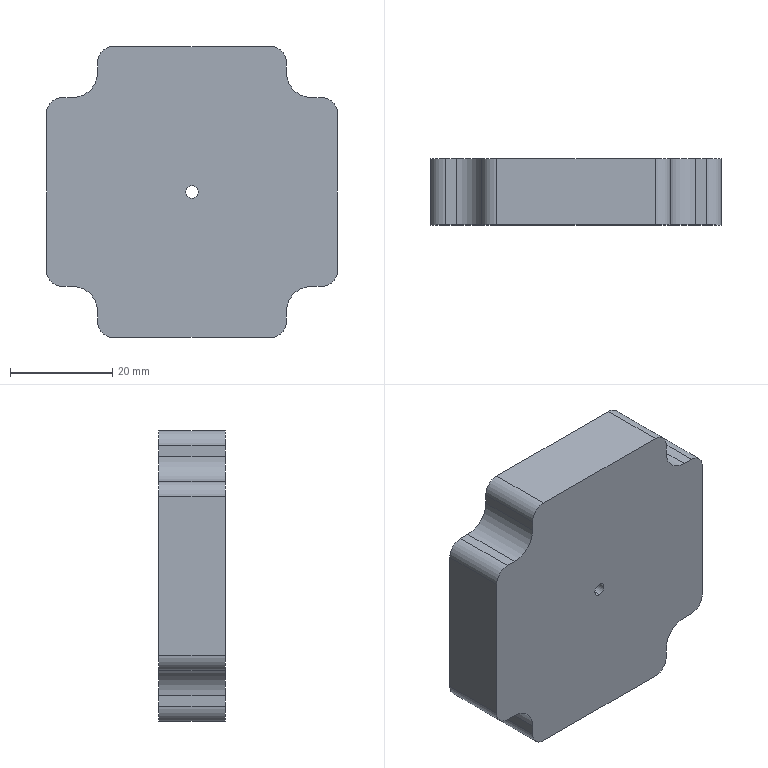Part | SolidWorks | features BaseBody 1 | 1 solid | 28 faces | box 57 x 13 x 57 mm | volume 37051 mm3 | cylinder 14 | plane 14 | commonest cylinder face diameters 6 x8 10 x4 2.5 x2
STEP:
#1=CARTESIAN_POINT('',(0.,0.,-1.25));
#2=VERTEX_POINT('',#1);
#3=CARTESIAN_POINT('',(0.,0.,1.25));
#4=VERTEX_POINT('',#3);
#5=CARTESIAN_POINT('',(0.,0.,0.));
#6=DIRECTION('',(0.,1.,0.));
#7=DIRECTION('',(0.,0.,1.));
#8=AXIS2_PLACEMENT_3D('',#5,#6,#7);
#9=CIRCLE('',#8,1.25);
#10=EDGE_CURVE('',#2,#4,#9,.T.);
#11=ORIENTED_EDGE('',*,*,#10,.F.);
#12=CARTESIAN_POINT('',(0.,13.,-1.25));
#13=VERTEX_POINT('',#12);
#14=CARTESIAN_POINT('',(0.,0.,-1.25));
#15=DIRECTION('',(0.,1.,0.));
#16=VECTOR('',#15,1000.);
#17=LINE('',#14,#16);
#18=EDGE_CURVE('',#2,#13,#17,.T.);
#19=ORIENTED_EDGE('',*,*,#18,.T.);
#20=CARTESIAN_POINT('',(0.,13.,1.25));
#21=VERTEX_POINT('',#20);
#22=CARTESIAN_POINT('',(0.,13.,0.));
#23=DIRECTION('',(0.,1.,0.));
#24=DIRECTION('',(0.,0.,1.));
#25=AXIS2_PLACEMENT_3D('',#22,#23,#24);
#26=CIRCLE('',#25,1.25);
#27=EDGE_CURVE('',#13,#21,#26,.T.);
#28=ORIENTED_EDGE('',*,*,#27,.T.);
#29=CARTESIAN_POINT('',(0.,0.,1.25));
#30=DIRECTION('',(0.,1.,0.));
#31=VECTOR('',#30,1000.);
#32=LINE('',#29,#31);
#33=EDGE_CURVE('',#4,#21,#32,.T.);
#34=ORIENTED_EDGE('',*,*,#33,.F.);
#35=EDGE_LOOP('',(#11,#19,#28,#34));
#36=FACE_OUTER_BOUND('',#35,.T.);
#37=CARTESIAN_POINT('',(0.,0.,0.));
#38=DIRECTION('',(0.,1.,0.));
#39=DIRECTION('',(0.,0.,1.));
#40=AXIS2_PLACEMENT_3D('',#37,#38,#39);
#41=CYLINDRICAL_SURFACE('',#40,1.25);
#42=ADVANCED_FACE('',(#36),#41,.F.);
#43=CARTESIAN_POINT('',(0.,13.,0.));
#44=DIRECTION('',(0.,1.,0.));
#45=DIRECTION('',(0.,0.,1.));
#46=AXIS2_PLACEMENT_3D('',#43,#44,#45);
#47=CIRCLE('',#46,1.25);
#48=EDGE_CURVE('',#21,#13,#47,.T.);
#49=ORIENTED_EDGE('',*,*,#48,.F.);
#50=ORIENTED_EDGE('',*,*,#27,.F.);
#51=EDGE_LOOP('',(#49,#50));
#52=FACE_BOUND('',#51,.T.);
#53=CARTESIAN_POINT('',(-18.5,13.,25.5));
#54=VERTEX_POINT('',#53);
#55=CARTESIAN_POINT('',(-18.5,13.,23.5));
#56=VERTEX_POINT('',#55);
#57=CARTESIAN_POINT('',(-18.5,13.,23.5));
#58=DIRECTION('',(0.,0.,-1.));
#59=VECTOR('',#58,1000.);
#60=LINE('',#57,#59);
#61=EDGE_CURVE('',#54,#56,#60,.T.);
#62=ORIENTED_EDGE('',*,*,#61,.F.);
#63=CARTESIAN_POINT('',(-15.5,13.,28.5));
#64=VERTEX_POINT('',#63);
#65=CARTESIAN_POINT('',(-15.5,13.,25.5));
#66=DIRECTION('',(0.,-1.,0.));
#67=DIRECTION('',(0.,0.,-1.));
#68=AXIS2_PLACEMENT_3D('',#65,#66,#67);
#69=CIRCLE('',#68,3.);
#70=EDGE_CURVE('',#64,#54,#69,.T.);
#71=ORIENTED_EDGE('',*,*,#70,.F.);
#72=CARTESIAN_POINT('',(15.5,13.,28.5));
#73=VERTEX_POINT('',#72);
#74=CARTESIAN_POINT('',(-23.5,13.,28.5));
#75=DIRECTION('',(-1.,0.,0.));
#76=VECTOR('',#75,1000.);
#77=LINE('',#74,#76);
#78=EDGE_CURVE('',#73,#64,#77,.T.);
#79=ORIENTED_EDGE('',*,*,#78,.F.);
#80=CARTESIAN_POINT('',(18.5,13.,25.5));
#81=VERTEX_POINT('',#80);
#82=CARTESIAN_POINT('',(15.5,13.,25.5));
#83=DIRECTION('',(0.,-1.,0.));
#84=DIRECTION('',(0.,0.,-1.));
#85=AXIS2_PLACEMENT_3D('',#82,#83,#84);
#86=CIRCLE('',#85,3.);
#87=EDGE_CURVE('',#81,#73,#86,.T.);
#88=ORIENTED_EDGE('',*,*,#87,.F.);
#89=CARTESIAN_POINT('',(18.5,13.,23.5));
#90=VERTEX_POINT('',#89);
#91=CARTESIAN_POINT('',(18.5,13.,23.5));
#92=DIRECTION('',(0.,0.,1.));
#93=VECTOR('',#92,1000.);
#94=LINE('',#91,#93);
#95=EDGE_CURVE('',#90,#81,#94,.T.);
#96=ORIENTED_EDGE('',*,*,#95,.F.);
#97=CARTESIAN_POINT('',(23.5,13.,18.5));
#98=VERTEX_POINT('',#97);
#99=CARTESIAN_POINT('',(23.5,13.,23.5));
#100=DIRECTION('',(0.,1.,0.));
#101=DIRECTION('',(0.,0.,-1.));
#102=AXIS2_PLACEMENT_3D('',#99,#100,#101);
#103=CIRCLE('',#102,5.);
#104=EDGE_CURVE('',#98,#90,#103,.T.);
#105=ORIENTED_EDGE('',*,*,#104,.F.);
#106=CARTESIAN_POINT('',(25.5,13.,18.5));
#107=VERTEX_POINT('',#106);
#108=CARTESIAN_POINT('',(-23.5,13.,18.5));
#109=DIRECTION('',(-1.,0.,0.));
#110=VECTOR('',#109,1000.);
#111=LINE('',#108,#110);
#112=EDGE_CURVE('',#107,#98,#111,.T.);
#113=ORIENTED_EDGE('',*,*,#112,.F.);
#114=CARTESIAN_POINT('',(28.5,13.,15.5));
#115=VERTEX_POINT('',#114);
#116=CARTESIAN_POINT('',(25.5,13.,15.5));
#117=DIRECTION('',(0.,-1.,0.));
#118=DIRECTION('',(0.,0.,-1.));
#119=AXIS2_PLACEMENT_3D('',#116,#117,#118);
#120=CIRCLE('',#119,3.);
#121=EDGE_CURVE('',#115,#107,#120,.T.);
#122=ORIENTED_EDGE('',*,*,#121,.F.);
#123=CARTESIAN_POINT('',(28.5,13.,-15.5));
#124=VERTEX_POINT('',#123);
#125=CARTESIAN_POINT('',(28.5,13.,23.5));
#126=DIRECTION('',(0.,0.,1.));
#127=VECTOR('',#126,1000.);
#128=LINE('',#125,#127);
#129=EDGE_CURVE('',#124,#115,#128,.T.);
#130=ORIENTED_EDGE('',*,*,#129,.F.);
#131=CARTESIAN_POINT('',(25.5,13.,-18.5));
#132=VERTEX_POINT('',#131);
#133=CARTESIAN_POINT('',(25.5,13.,-15.5));
#134=DIRECTION('',(0.,-1.,0.));
#135=DIRECTION('',(0.,0.,-1.));
#136=AXIS2_PLACEMENT_3D('',#133,#134,#135);
#137=CIRCLE('',#136,3.);
#138=EDGE_CURVE('',#132,#124,#137,.T.);
#139=ORIENTED_EDGE('',*,*,#138,.F.);
#140=CARTESIAN_POINT('',(23.5,13.,-18.5));
#141=VERTEX_POINT('',#140);
#142=CARTESIAN_POINT('',(-23.5,13.,-18.5));
#143=DIRECTION('',(1.,0.,0.));
#144=VECTOR('',#143,1000.);
#145=LINE('',#142,#144);
#146=EDGE_CURVE('',#141,#132,#145,.T.);
#147=ORIENTED_EDGE('',*,*,#146,.F.);
#148=CARTESIAN_POINT('',(18.5,13.,-23.5));
#149=VERTEX_POINT('',#148);
#150=CARTESIAN_POINT('',(23.5,13.,-23.5));
#151=DIRECTION('',(0.,1.,0.));
#152=DIRECTION('',(0.,0.,-1.));
#153=AXIS2_PLACEMENT_3D('',#150,#151,#152);
#154=CIRCLE('',#153,5.);
#155=EDGE_CURVE('',#149,#141,#154,.T.);
#156=ORIENTED_EDGE('',*,*,#155,.F.);
#157=CARTESIAN_POINT('',(18.5,13.,-25.5));
#158=VERTEX_POINT('',#157);
#159=CARTESIAN_POINT('',(18.5,13.,23.5));
#160=DIRECTION('',(0.,0.,1.));
#161=VECTOR('',#160,1000.);
#162=LINE('',#159,#161);
#163=EDGE_CURVE('',#158,#149,#162,.T.);
#164=ORIENTED_EDGE('',*,*,#163,.F.);
#165=CARTESIAN_POINT('',(15.5,13.,-28.5));
#166=VERTEX_POINT('',#165);
#167=CARTESIAN_POINT('',(15.5,13.,-25.5));
#168=DIRECTION('',(0.,-1.,0.));
#169=DIRECTION('',(0.,0.,-1.));
#170=AXIS2_PLACEMENT_3D('',#167,#168,#169);
#171=CIRCLE('',#170,3.);
#172=EDGE_CURVE('',#166,#158,#171,.T.);
#173=ORIENTED_EDGE('',*,*,#172,.F.);
#174=CARTESIAN_POINT('',(-15.5,13.,-28.5));
#175=VERTEX_POINT('',#174);
#176=CARTESIAN_POINT('',(-23.5,13.,-28.5));
#177=DIRECTION('',(1.,0.,0.));
#178=VECTOR('',#177,1000.);
#179=LINE('',#176,#178);
#180=EDGE_CURVE('',#175,#166,#179,.T.);
#181=ORIENTED_EDGE('',*,*,#180,.F.);
#182=CARTESIAN_POINT('',(-18.5,13.,-25.5));
#183=VERTEX_POINT('',#182);
#184=CARTESIAN_POINT('',(-15.5,13.,-25.5));
#185=DIRECTION('',(0.,-1.,0.));
#186=DIRECTION('',(0.,0.,-1.));
#187=AXIS2_PLACEMENT_3D('',#184,#185,#186);
#188=CIRCLE('',#187,3.);
#189=EDGE_CURVE('',#183,#175,#188,.T.);
#190=ORIENTED_EDGE('',*,*,#189,.F.);
#191=CARTESIAN_POINT('',(-18.5,13.,-23.5));
#192=VERTEX_POINT('',#191);
#193=CARTESIAN_POINT('',(-18.5,13.,23.5));
#194=DIRECTION('',(0.,0.,-1.));
#195=VECTOR('',#194,1000.);
#196=LINE('',#193,#195);
#197=EDGE_CURVE('',#192,#183,#196,.T.);
#198=ORIENTED_EDGE('',*,*,#197,.F.);
#199=CARTESIAN_POINT('',(-23.5,13.,-18.5));
#200=VERTEX_POINT('',#199);
#201=CARTESIAN_POINT('',(-23.5,13.,-23.5));
#202=DIRECTION('',(0.,1.,0.));
#203=DIRECTION('',(0.,0.,-1.));
#204=AXIS2_PLACEMENT_3D('',#201,#202,#203);
#205=CIRCLE('',#204,5.);
#206=EDGE_CURVE('',#200,#192,#205,.T.);
#207=ORIENTED_EDGE('',*,*,#206,.F.);
#208=CARTESIAN_POINT('',(-25.5,13.,-18.5));
#209=VERTEX_POINT('',#208);
#210=CARTESIAN_POINT('',(-23.5,13.,-18.5));
#211=DIRECTION('',(1.,0.,0.));
#212=VECTOR('',#211,1000.);
#213=LINE('',#210,#212);
#214=EDGE_CURVE('',#209,#200,#213,.T.);
#215=ORIENTED_EDGE('',*,*,#214,.F.);
#216=CARTESIAN_POINT('',(-28.5,13.,-15.5));
#217=VERTEX_POINT('',#216);
#218=CARTESIAN_POINT('',(-25.5,13.,-15.5));
#219=DIRECTION('',(0.,-1.,0.));
#220=DIRECTION('',(0.,0.,-1.));
#221=AXIS2_PLACEMENT_3D('',#218,#219,#220);
#222=CIRCLE('',#221,3.);
#223=EDGE_CURVE('',#217,#209,#222,.T.);
#224=ORIENTED_EDGE('',*,*,#223,.F.);
#225=CARTESIAN_POINT('',(-28.5,13.,15.5));
#226=VERTEX_POINT('',#225);
#227=CARTESIAN_POINT('',(-28.5,13.,23.5));
#228=DIRECTION('',(0.,0.,-1.));
#229=VECTOR('',#228,1000.);
#230=LINE('',#227,#229);
#231=EDGE_CURVE('',#226,#217,#230,.T.);
#232=ORIENTED_EDGE('',*,*,#231,.F.);
#233=CARTESIAN_POINT('',(-25.5,13.,18.5));
#234=VERTEX_POINT('',#233);
#235=CARTESIAN_POINT('',(-25.5,13.,15.5));
#236=DIRECTION('',(0.,-1.,0.));
#237=DIRECTION('',(0.,0.,-1.));
#238=AXIS2_PLACEMENT_3D('',#235,#236,#237);
#239=CIRCLE('',#238,3.);
#240=EDGE_CURVE('',#234,#226,#239,.T.);
#241=ORIENTED_EDGE('',*,*,#240,.F.);
#242=CARTESIAN_POINT('',(-23.5,13.,18.5));
#243=VERTEX_POINT('',#242);
#244=CARTESIAN_POINT('',(-23.5,13.,18.5));
#245=DIRECTION('',(-1.,0.,0.));
#246=VECTOR('',#245,1000.);
#247=LINE('',#244,#246);
#248=EDGE_CURVE('',#243,#234,#247,.T.);
#249=ORIENTED_EDGE('',*,*,#248,.F.);
#250=CARTESIAN_POINT('',(-23.5,13.,23.5));
#251=DIRECTION('',(0.,1.,0.));
#252=DIRECTION('',(0.,0.,-1.));
#253=AXIS2_PLACEMENT_3D('',#250,#251,#252);
#254=CIRCLE('',#253,5.);
#255=EDGE_CURVE('',#56,#243,#254,.T.);
#256=ORIENTED_EDGE('',*,*,#255,.F.);
#257=EDGE_LOOP('',(#62,#71,#79,#88,#96,#105,#113,#122,#130,#139,#147,#156,#164,#173,#181,#190,#198,#207,#215,#224,#232,#241,#249,#256));
#258=FACE_OUTER_BOUND('',#257,.T.);
#259=CARTESIAN_POINT('',(-23.5,13.,23.5));
#260=DIRECTION('',(0.,-1.,0.));
#261=DIRECTION('',(0.,0.,-1.));
#262=AXIS2_PLACEMENT_3D('',#259,#260,#261);
#263=PLANE('',#262);
#264=ADVANCED_FACE('',(#52,#258),#263,.F.);
#265=CARTESIAN_POINT('',(-18.5,0.,23.5));
#266=VERTEX_POINT('',#265);
#267=CARTESIAN_POINT('',(-18.5,13.,23.5));
#268=DIRECTION('',(0.,-1.,0.));
#269=VECTOR('',#268,1000.);
#270=LINE('',#267,#269);
#271=EDGE_CURVE('',#56,#266,#270,.T.);
#272=ORIENTED_EDGE('',*,*,#271,.F.);
#273=ORIENTED_EDGE('',*,*,#255,.T.);
#274=CARTESIAN_POINT('',(-23.5,0.,18.5));
#275=VERTEX_POINT('',#274);
#276=CARTESIAN_POINT('',(-23.5,13.,18.5));
#277=DIRECTION('',(0.,1.,0.));
#278=VECTOR('',#277,1000.);
#279=LINE('',#276,#278);
#280=EDGE_CURVE('',#275,#243,#279,.T.);
#281=ORIENTED_EDGE('',*,*,#280,.F.);
#282=CARTESIAN_POINT('',(-23.5,0.,23.5));
#283=DIRECTION('',(0.,1.,0.));
#284=DIRECTION('',(0.,0.,-1.));
#285=AXIS2_PLACEMENT_3D('',#282,#283,#284);
#286=CIRCLE('',#285,5.);
#287=EDGE_CURVE('',#266,#275,#286,.T.);
#288=ORIENTED_EDGE('',*,*,#287,.F.);
#289=EDGE_LOOP('',(#272,#273,#281,#288));
#290=FACE_OUTER_BOUND('',#289,.T.);
#291=CARTESIAN_POINT('',(-23.5,13.,23.5));
#292=DIRECTION('',(0.,-1.,0.));
#293=DIRECTION('',(0.,0.,-1.));
#294=AXIS2_PLACEMENT_3D('',#291,#292,#293);
#295=CYLINDRICAL_SURFACE('',#294,5.);
#296=ADVANCED_FACE('',(#290),#295,.F.);
#297=CARTESIAN_POINT('',(-18.5,0.,25.5));
#298=VERTEX_POINT('',#297);
#299=CARTESIAN_POINT('',(-18.5,13.,25.5));
#300=DIRECTION('',(0.,-1.,0.));
#301=VECTOR('',#300,1000.);
#302=LINE('',#299,#301);
#303=EDGE_CURVE('',#54,#298,#302,.T.);
#304=ORIENTED_EDGE('',*,*,#303,.F.);
#305=ORIENTED_EDGE('',*,*,#61,.T.);
#306=ORIENTED_EDGE('',*,*,#271,.T.);
#307=CARTESIAN_POINT('',(-18.5,0.,23.5));
#308=DIRECTION('',(0.,0.,-1.));
#309=VECTOR('',#308,1000.);
#310=LINE('',#307,#309);
#311=EDGE_CURVE('',#298,#266,#310,.T.);
#312=ORIENTED_EDGE('',*,*,#311,.F.);
#313=EDGE_LOOP('',(#304,#305,#306,#312));
#314=FACE_OUTER_BOUND('',#313,.T.);
#315=CARTESIAN_POINT('',(-18.5,13.,23.5));
#316=DIRECTION('',(1.,0.,0.));
#317=DIRECTION('',(0.,1.,0.));
#318=AXIS2_PLACEMENT_3D('',#315,#316,#317);
#319=PLANE('',#318);
#320=ADVANCED_FACE('',(#314),#319,.F.);
#321=ORIENTED_EDGE('',*,*,#70,.T.);
#322=ORIENTED_EDGE('',*,*,#303,.T.);
#323=CARTESIAN_POINT('',(-15.5,0.,28.5));
#324=VERTEX_POINT('',#323);
#325=CARTESIAN_POINT('',(-15.5,0.,25.5));
#326=DIRECTION('',(0.,1.,0.));
#327=DIRECTION('',(0.,0.,-1.));
#328=AXIS2_PLACEMENT_3D('',#325,#326,#327);
#329=CIRCLE('',#328,3.);
#330=EDGE_CURVE('',#298,#324,#329,.T.);
#331=ORIENTED_EDGE('',*,*,#330,.T.);
#332=CARTESIAN_POINT('',(-15.5,13.,28.5));
#333=DIRECTION('',(0.,1.,0.));
#334=VECTOR('',#333,1000.);
#335=LINE('',#332,#334);
#336=EDGE_CURVE('',#324,#64,#335,.T.);
#337=ORIENTED_EDGE('',*,*,#336,.T.);
#338=EDGE_LOOP('',(#321,#322,#331,#337));
#339=FACE_OUTER_BOUND('',#338,.T.);
#340=CARTESIAN_POINT('',(-15.5,13.,25.5));
#341=DIRECTION('',(0.,-1.,0.));
#342=DIRECTION('',(0.,0.,-1.));
#343=AXIS2_PLACEMENT_3D('',#340,#341,#342);
#344=CYLINDRICAL_SURFACE('',#343,3.);
#345=ADVANCED_FACE('',(#339),#344,.T.);
#346=CARTESIAN_POINT('',(15.5,0.,28.5));
#347=VERTEX_POINT('',#346);
#348=CARTESIAN_POINT('',(15.5,13.,28.5));
#349=DIRECTION('',(0.,-1.,0.));
#350=VECTOR('',#349,1000.);
#351=LINE('',#348,#350);
#352=EDGE_CURVE('',#73,#347,#351,.T.);
#353=ORIENTED_EDGE('',*,*,#352,.F.);
#354=ORIENTED_EDGE('',*,*,#78,.T.);
#355=ORIENTED_EDGE('',*,*,#336,.F.);
#356=CARTESIAN_POINT('',(-15.5,0.,28.5));
#357=DIRECTION('',(-1.,0.,0.));
#358=VECTOR('',#357,1000.);
#359=LINE('',#356,#358);
#360=EDGE_CURVE('',#347,#324,#359,.T.);
#361=ORIENTED_EDGE('',*,*,#360,.F.);
#362=EDGE_LOOP('',(#353,#354,#355,#361));
#363=FACE_OUTER_BOUND('',#362,.T.);
#364=CARTESIAN_POINT('',(-15.5,13.,28.5));
#365=DIRECTION('',(0.,0.,-1.));
#366=DIRECTION('',(0.,-1.,0.));
#367=AXIS2_PLACEMENT_3D('',#364,#365,#366);
#368=PLANE('',#367);
#369=ADVANCED_FACE('',(#363),#368,.F.);
#370=ORIENTED_EDGE('',*,*,#87,.T.);
#371=ORIENTED_EDGE('',*,*,#352,.T.);
#372=CARTESIAN_POINT('',(18.5,0.,25.5));
#373=VERTEX_POINT('',#372);
#374=CARTESIAN_POINT('',(15.5,0.,25.5));
#375=DIRECTION('',(0.,1.,0.));
#376=DIRECTION('',(0.,0.,-1.));
#377=AXIS2_PLACEMENT_3D('',#374,#375,#376);
#378=CIRCLE('',#377,3.);
#379=EDGE_CURVE('',#347,#373,#378,.T.);
#380=ORIENTED_EDGE('',*,*,#379,.T.);
#381=CARTESIAN_POINT('',(18.5,13.,25.5));
#382=DIRECTION('',(0.,1.,0.));
#383=VECTOR('',#382,1000.);
#384=LINE('',#381,#383);
#385=EDGE_CURVE('',#373,#81,#384,.T.);
#386=ORIENTED_EDGE('',*,*,#385,.T.);
#387=EDGE_LOOP('',(#370,#371,#380,#386));
#388=FACE_OUTER_BOUND('',#387,.T.);
#389=CARTESIAN_POINT('',(15.5,13.,25.5));
#390=DIRECTION('',(0.,-1.,0.));
#391=DIRECTION('',(0.,0.,-1.));
#392=AXIS2_PLACEMENT_3D('',#389,#390,#391);
#393=CYLINDRICAL_SURFACE('',#392,3.);
#394=ADVANCED_FACE('',(#388),#393,.T.);
#395=CARTESIAN_POINT('',(18.5,0.,23.5));
#396=VERTEX_POINT('',#395);
#397=CARTESIAN_POINT('',(18.5,13.,23.5));
#398=DIRECTION('',(0.,-1.,0.));
#399=VECTOR('',#398,1000.);
#400=LINE('',#397,#399);
#401=EDGE_CURVE('',#90,#396,#400,.T.);
#402=ORIENTED_EDGE('',*,*,#401,.F.);
#403=ORIENTED_EDGE('',*,*,#95,.T.);
#404=ORIENTED_EDGE('',*,*,#385,.F.);
#405=CARTESIAN_POINT('',(18.5,0.,25.5));
#406=DIRECTION('',(0.,0.,1.));
#407=VECTOR('',#406,1000.);
#408=LINE('',#405,#407);
#409=EDGE_CURVE('',#396,#373,#408,.T.);
#410=ORIENTED_EDGE('',*,*,#409,.F.);
#411=EDGE_LOOP('',(#402,#403,#404,#410));
#412=FACE_OUTER_BOUND('',#411,.T.);
#413=CARTESIAN_POINT('',(18.5,13.,25.5));
#414=DIRECTION('',(-1.,0.,0.));
#415=DIRECTION('',(0.,0.,1.));
#416=AXIS2_PLACEMENT_3D('',#413,#414,#415);
#417=PLANE('',#416);
#418=ADVANCED_FACE('',(#412),#417,.F.);
#419=CARTESIAN_POINT('',(23.5,0.,18.5));
#420=VERTEX_POINT('',#419);
#421=CARTESIAN_POINT('',(23.5,13.,18.5));
#422=DIRECTION('',(0.,-1.,0.));
#423=VECTOR('',#422,1000.);
#424=LINE('',#421,#423);
#425=EDGE_CURVE('',#98,#420,#424,.T.);
#426=ORIENTED_EDGE('',*,*,#425,.F.);
#427=ORIENTED_EDGE('',*,*,#104,.T.);
#428=ORIENTED_EDGE('',*,*,#401,.T.);
#429=CARTESIAN_POINT('',(23.5,0.,23.5));
#430=DIRECTION('',(0.,1.,0.));
#431=DIRECTION('',(0.,0.,-1.));
#432=AXIS2_PLACEMENT_3D('',#429,#430,#431);
#433=CIRCLE('',#432,5.);
#434=EDGE_CURVE('',#420,#396,#433,.T.);
#435=ORIENTED_EDGE('',*,*,#434,.F.);
#436=EDGE_LOOP('',(#426,#427,#428,#435));
#437=FACE_OUTER_BOUND('',#436,.T.);
#438=CARTESIAN_POINT('',(23.5,13.,23.5));
#439=DIRECTION('',(0.,-1.,0.));
#440=DIRECTION('',(0.,0.,-1.));
#441=AXIS2_PLACEMENT_3D('',#438,#439,#440);
#442=CYLINDRICAL_SURFACE('',#441,5.);
#443=ADVANCED_FACE('',(#437),#442,.F.);
#444=CARTESIAN_POINT('',(25.5,0.,18.5));
#445=VERTEX_POINT('',#444);
#446=CARTESIAN_POINT('',(25.5,13.,18.5));
#447=DIRECTION('',(0.,-1.,0.));
#448=VECTOR('',#447,1000.);
#449=LINE('',#446,#448);
#450=EDGE_CURVE('',#107,#445,#449,.T.);
#451=ORIENTED_EDGE('',*,*,#450,.F.);
#452=ORIENTED_EDGE('',*,*,#112,.T.);
#453=ORIENTED_EDGE('',*,*,#425,.T.);
#454=CARTESIAN_POINT('',(23.5,0.,18.5));
#455=DIRECTION('',(-1.,0.,0.));
#456=VECTOR('',#455,1000.);
#457=LINE('',#454,#456);
#458=EDGE_CURVE('',#445,#420,#457,.T.);
#459=ORIENTED_EDGE('',*,*,#458,.F.);
#460=EDGE_LOOP('',(#451,#452,#453,#459));
#461=FACE_OUTER_BOUND('',#460,.T.);
#462=CARTESIAN_POINT('',(23.5,13.,18.5));
#463=DIRECTION('',(0.,0.,-1.));
#464=DIRECTION('',(0.,-1.,0.));
#465=AXIS2_PLACEMENT_3D('',#462,#463,#464);
#466=PLANE('',#465);
#467=ADVANCED_FACE('',(#461),#466,.F.);
#468=ORIENTED_EDGE('',*,*,#121,.T.);
#469=ORIENTED_EDGE('',*,*,#450,.T.);
#470=CARTESIAN_POINT('',(28.5,0.,15.5));
#471=VERTEX_POINT('',#470);
#472=CARTESIAN_POINT('',(25.5,0.,15.5));
#473=DIRECTION('',(0.,1.,0.));
#474=DIRECTION('',(0.,0.,-1.));
#475=AXIS2_PLACEMENT_3D('',#472,#473,#474);
#476=CIRCLE('',#475,3.);
#477=EDGE_CURVE('',#445,#471,#476,.T.);
#478=ORIENTED_EDGE('',*,*,#477,.T.);
#479=CARTESIAN_POINT('',(28.5,13.,15.5));
#480=DIRECTION('',(0.,1.,0.));
#481=VECTOR('',#480,1000.);
#482=LINE('',#479,#481);
#483=EDGE_CURVE('',#471,#115,#482,.T.);
#484=ORIENTED_EDGE('',*,*,#483,.T.);
#485=EDGE_LOOP('',(#468,#469,#478,#484));
#486=FACE_OUTER_BOUND('',#485,.T.);
#487=CARTESIAN_POINT('',(25.5,13.,15.5));
#488=DIRECTION('',(0.,-1.,0.));
#489=DIRECTION('',(0.,0.,-1.));
#490=AXIS2_PLACEMENT_3D('',#487,#488,#489);
#491=CYLINDRICAL_SURFACE('',#490,3.);
#492=ADVANCED_FACE('',(#486),#491,.T.);
#493=CARTESIAN_POINT('',(28.5,0.,-15.5));
#494=VERTEX_POINT('',#493);
#495=CARTESIAN_POINT('',(28.5,13.,-15.5));
#496=DIRECTION('',(0.,-1.,0.));
#497=VECTOR('',#496,1000.);
#498=LINE('',#495,#497);
#499=EDGE_CURVE('',#124,#494,#498,.T.);
#500=ORIENTED_EDGE('',*,*,#499,.F.);
#501=ORIENTED_EDGE('',*,*,#129,.T.);
#502=ORIENTED_EDGE('',*,*,#483,.F.);
#503=CARTESIAN_POINT('',(28.5,0.,15.5));
#504=DIRECTION('',(0.,0.,1.));
#505=VECTOR('',#504,1000.);
#506=LINE('',#503,#505);
#507=EDGE_CURVE('',#494,#471,#506,.T.);
#508=ORIENTED_EDGE('',*,*,#507,.F.);
#509=EDGE_LOOP('',(#500,#501,#502,#508));
#510=FACE_OUTER_BOUND('',#509,.T.);
#511=CARTESIAN_POINT('',(28.5,13.,15.5));
#512=DIRECTION('',(-1.,0.,0.));
#513=DIRECTION('',(0.,1.,0.));
#514=AXIS2_PLACEMENT_3D('',#511,#512,#513);
#515=PLANE('',#514);
#516=ADVANCED_FACE('',(#510),#515,.F.);
#517=ORIENTED_EDGE('',*,*,#138,.T.);
#518=ORIENTED_EDGE('',*,*,#499,.T.);
#519=CARTESIAN_POINT('',(25.5,0.,-18.5));
#520=VERTEX_POINT('',#519);
#521=CARTESIAN_POINT('',(25.5,0.,-15.5));
#522=DIRECTION('',(0.,1.,0.));
#523=DIRECTION('',(0.,0.,-1.));
#524=AXIS2_PLACEMENT_3D('',#521,#522,#523);
#525=CIRCLE('',#524,3.);
#526=EDGE_CURVE('',#494,#520,#525,.T.);
#527=ORIENTED_EDGE('',*,*,#526,.T.);
#528=CARTESIAN_POINT('',(25.5,13.,-18.5));
#529=DIRECTION('',(0.,1.,0.));
#530=VECTOR('',#529,1000.);
#531=LINE('',#528,#530);
#532=EDGE_CURVE('',#520,#132,#531,.T.);
#533=ORIENTED_EDGE('',*,*,#532,.T.);
#534=EDGE_LOOP('',(#517,#518,#527,#533));
#535=FACE_OUTER_BOUND('',#534,.T.);
#536=CARTESIAN_POINT('',(25.5,13.,-15.5));
#537=DIRECTION('',(0.,-1.,0.));
#538=DIRECTION('',(0.,0.,-1.));
#539=AXIS2_PLACEMENT_3D('',#536,#537,#538);
#540=CYLINDRICAL_SURFACE('',#539,3.);
#541=ADVANCED_FACE('',(#535),#540,.T.);
#542=CARTESIAN_POINT('',(23.5,0.,-18.5));
#543=VERTEX_POINT('',#542);
#544=CARTESIAN_POINT('',(23.5,13.,-18.5));
#545=DIRECTION('',(0.,-1.,0.));
#546=VECTOR('',#545,1000.);
#547=LINE('',#544,#546);
#548=EDGE_CURVE('',#141,#543,#547,.T.);
#549=ORIENTED_EDGE('',*,*,#548,.F.);
#550=ORIENTED_EDGE('',*,*,#146,.T.);
#551=ORIENTED_EDGE('',*,*,#532,.F.);
#552=CARTESIAN_POINT('',(25.5,0.,-18.5));
#553=DIRECTION('',(1.,0.,0.));
#554=VECTOR('',#553,1000.);
#555=LINE('',#552,#554);
#556=EDGE_CURVE('',#543,#520,#555,.T.);
#557=ORIENTED_EDGE('',*,*,#556,.F.);
#558=EDGE_LOOP('',(#549,#550,#551,#557));
#559=FACE_OUTER_BOUND('',#558,.T.);
#560=CARTESIAN_POINT('',(25.5,13.,-18.5));
#561=DIRECTION('',(0.,0.,1.));
#562=DIRECTION('',(1.,0.,0.));
#563=AXIS2_PLACEMENT_3D('',#560,#561,#562);
#564=PLANE('',#563);
#565=ADVANCED_FACE('',(#559),#564,.F.);
#566=CARTESIAN_POINT('',(18.5,0.,-23.5));
#567=VERTEX_POINT('',#566);
#568=CARTESIAN_POINT('',(18.5,13.,-23.5));
#569=DIRECTION('',(0.,-1.,0.));
#570=VECTOR('',#569,1000.);
#571=LINE('',#568,#570);
#572=EDGE_CURVE('',#149,#567,#571,.T.);
#573=ORIENTED_EDGE('',*,*,#572,.F.);
#574=ORIENTED_EDGE('',*,*,#155,.T.);
#575=ORIENTED_EDGE('',*,*,#548,.T.);
#576=CARTESIAN_POINT('',(23.5,0.,-23.5));
#577=DIRECTION('',(0.,1.,0.));
#578=DIRECTION('',(0.,0.,-1.));
#579=AXIS2_PLACEMENT_3D('',#576,#577,#578);
#580=CIRCLE('',#579,5.);
#581=EDGE_CURVE('',#567,#543,#580,.T.);
#582=ORIENTED_EDGE('',*,*,#581,.F.);
#583=EDGE_LOOP('',(#573,#574,#575,#582));
#584=FACE_OUTER_BOUND('',#583,.T.);
#585=CARTESIAN_POINT('',(23.5,13.,-23.5));
#586=DIRECTION('',(0.,-1.,0.));
#587=DIRECTION('',(0.,0.,-1.));
#588=AXIS2_PLACEMENT_3D('',#585,#586,#587);
#589=CYLINDRICAL_SURFACE('',#588,5.);
#590=ADVANCED_FACE('',(#584),#589,.F.);
#591=CARTESIAN_POINT('',(18.5,0.,-25.5));
#592=VERTEX_POINT('',#591);
#593=CARTESIAN_POINT('',(18.5,13.,-25.5));
#594=DIRECTION('',(0.,-1.,0.));
#595=VECTOR('',#594,1000.);
#596=LINE('',#593,#595);
#597=EDGE_CURVE('',#158,#592,#596,.T.);
#598=ORIENTED_EDGE('',*,*,#597,.F.);
#599=ORIENTED_EDGE('',*,*,#163,.T.);
#600=ORIENTED_EDGE('',*,*,#572,.T.);
#601=CARTESIAN_POINT('',(18.5,0.,-23.5));
#602=DIRECTION('',(0.,0.,1.));
#603=VECTOR('',#602,1000.);
#604=LINE('',#601,#603);
#605=EDGE_CURVE('',#592,#567,#604,.T.);
#606=ORIENTED_EDGE('',*,*,#605,.F.);
#607=EDGE_LOOP('',(#598,#599,#600,#606));
#608=FACE_OUTER_BOUND('',#607,.T.);
#609=CARTESIAN_POINT('',(18.5,13.,-23.5));
#610=DIRECTION('',(-1.,0.,0.));
#611=DIRECTION('',(0.,0.,1.));
#612=AXIS2_PLACEMENT_3D('',#609,#610,#611);
#613=PLANE('',#612);
#614=ADVANCED_FACE('',(#608),#613,.F.);
#615=ORIENTED_EDGE('',*,*,#172,.T.);
#616=ORIENTED_EDGE('',*,*,#597,.T.);
#617=CARTESIAN_POINT('',(15.5,0.,-28.5));
#618=VERTEX_POINT('',#617);
#619=CARTESIAN_POINT('',(15.5,0.,-25.5));
#620=DIRECTION('',(0.,1.,0.));
#621=DIRECTION('',(0.,0.,-1.));
#622=AXIS2_PLACEMENT_3D('',#619,#620,#621);
#623=CIRCLE('',#622,3.);
#624=EDGE_CURVE('',#592,#618,#623,.T.);
#625=ORIENTED_EDGE('',*,*,#624,.T.);
#626=CARTESIAN_POINT('',(15.5,13.,-28.5));
#627=DIRECTION('',(0.,1.,0.));
#628=VECTOR('',#627,1000.);
#629=LINE('',#626,#628);
#630=EDGE_CURVE('',#618,#166,#629,.T.);
#631=ORIENTED_EDGE('',*,*,#630,.T.);
#632=EDGE_LOOP('',(#615,#616,#625,#631));
#633=FACE_OUTER_BOUND('',#632,.T.);
#634=CARTESIAN_POINT('',(15.5,13.,-25.5));
#635=DIRECTION('',(0.,-1.,0.));
#636=DIRECTION('',(0.,0.,-1.));
#637=AXIS2_PLACEMENT_3D('',#634,#635,#636);
#638=CYLINDRICAL_SURFACE('',#637,3.);
#639=ADVANCED_FACE('',(#633),#638,.T.);
#640=CARTESIAN_POINT('',(-15.5,0.,-28.5));
#641=VERTEX_POINT('',#640);
#642=CARTESIAN_POINT('',(-15.5,13.,-28.5));
#643=DIRECTION('',(0.,-1.,0.));
#644=VECTOR('',#643,1000.);
#645=LINE('',#642,#644);
#646=EDGE_CURVE('',#175,#641,#645,.T.);
#647=ORIENTED_EDGE('',*,*,#646,.F.);
#648=ORIENTED_EDGE('',*,*,#180,.T.);
#649=ORIENTED_EDGE('',*,*,#630,.F.);
#650=CARTESIAN_POINT('',(15.5,0.,-28.5));
#651=DIRECTION('',(1.,0.,0.));
#652=VECTOR('',#651,1000.);
#653=LINE('',#650,#652);
#654=EDGE_CURVE('',#641,#618,#653,.T.);
#655=ORIENTED_EDGE('',*,*,#654,.F.);
#656=EDGE_LOOP('',(#647,#648,#649,#655));
#657=FACE_OUTER_BOUND('',#656,.T.);
#658=CARTESIAN_POINT('',(15.5,13.,-28.5));
#659=DIRECTION('',(0.,0.,1.));
#660=DIRECTION('',(1.,0.,0.));
#661=AXIS2_PLACEMENT_3D('',#658,#659,#660);
#662=PLANE('',#661);
#663=ADVANCED_FACE('',(#657),#662,.F.);
#664=ORIENTED_EDGE('',*,*,#189,.T.);
#665=ORIENTED_EDGE('',*,*,#646,.T.);
#666=CARTESIAN_POINT('',(-18.5,0.,-25.5));
#667=VERTEX_POINT('',#666);
#668=CARTESIAN_POINT('',(-15.5,0.,-25.5));
#669=DIRECTION('',(0.,1.,0.));
#670=DIRECTION('',(0.,0.,-1.));
#671=AXIS2_PLACEMENT_3D('',#668,#669,#670);
#672=CIRCLE('',#671,3.);
#673=EDGE_CURVE('',#641,#667,#672,.T.);
#674=ORIENTED_EDGE('',*,*,#673,.T.);
#675=CARTESIAN_POINT('',(-18.5,13.,-25.5));
#676=DIRECTION('',(0.,1.,0.));
#677=VECTOR('',#676,1000.);
#678=LINE('',#675,#677);
#679=EDGE_CURVE('',#667,#183,#678,.T.);
#680=ORIENTED_EDGE('',*,*,#679,.T.);
#681=EDGE_LOOP('',(#664,#665,#674,#680));
#682=FACE_OUTER_BOUND('',#681,.T.);
#683=CARTESIAN_POINT('',(-15.5,13.,-25.5));
#684=DIRECTION('',(0.,-1.,0.));
#685=DIRECTION('',(0.,0.,-1.));
#686=AXIS2_PLACEMENT_3D('',#683,#684,#685);
#687=CYLINDRICAL_SURFACE('',#686,3.);
#688=ADVANCED_FACE('',(#682),#687,.T.);
#689=CARTESIAN_POINT('',(-18.5,0.,-23.5));
#690=VERTEX_POINT('',#689);
#691=CARTESIAN_POINT('',(-18.5,13.,-23.5));
#692=DIRECTION('',(0.,-1.,0.));
#693=VECTOR('',#692,1000.);
#694=LINE('',#691,#693);
#695=EDGE_CURVE('',#192,#690,#694,.T.);
#696=ORIENTED_EDGE('',*,*,#695,.F.);
#697=ORIENTED_EDGE('',*,*,#197,.T.);
#698=ORIENTED_EDGE('',*,*,#679,.F.);
#699=CARTESIAN_POINT('',(-18.5,0.,-25.5));
#700=DIRECTION('',(0.,0.,-1.));
#701=VECTOR('',#700,1000.);
#702=LINE('',#699,#701);
#703=EDGE_CURVE('',#690,#667,#702,.T.);
#704=ORIENTED_EDGE('',*,*,#703,.F.);
#705=EDGE_LOOP('',(#696,#697,#698,#704));
#706=FACE_OUTER_BOUND('',#705,.T.);
#707=CARTESIAN_POINT('',(-18.5,13.,-25.5));
#708=DIRECTION('',(1.,0.,0.));
#709=DIRECTION('',(0.,1.,0.));
#710=AXIS2_PLACEMENT_3D('',#707,#708,#709);
#711=PLANE('',#710);
#712=ADVANCED_FACE('',(#706),#711,.F.);
#713=CARTESIAN_POINT('',(-23.5,0.,-18.5));
#714=VERTEX_POINT('',#713);
#715=CARTESIAN_POINT('',(-23.5,13.,-18.5));
#716=DIRECTION('',(0.,-1.,0.));
#717=VECTOR('',#716,1000.);
#718=LINE('',#715,#717);
#719=EDGE_CURVE('',#200,#714,#718,.T.);
#720=ORIENTED_EDGE('',*,*,#719,.F.);
#721=ORIENTED_EDGE('',*,*,#206,.T.);
#722=ORIENTED_EDGE('',*,*,#695,.T.);
#723=CARTESIAN_POINT('',(-23.5,0.,-23.5));
#724=DIRECTION('',(0.,1.,0.));
#725=DIRECTION('',(0.,0.,-1.));
#726=AXIS2_PLACEMENT_3D('',#723,#724,#725);
#727=CIRCLE('',#726,5.);
#728=EDGE_CURVE('',#714,#690,#727,.T.);
#729=ORIENTED_EDGE('',*,*,#728,.F.);
#730=EDGE_LOOP('',(#720,#721,#722,#729));
#731=FACE_OUTER_BOUND('',#730,.T.);
#732=CARTESIAN_POINT('',(-23.5,13.,-23.5));
#733=DIRECTION('',(0.,-1.,0.));
#734=DIRECTION('',(0.,0.,-1.));
#735=AXIS2_PLACEMENT_3D('',#732,#733,#734);
#736=CYLINDRICAL_SURFACE('',#735,5.);
#737=ADVANCED_FACE('',(#731),#736,.F.);
#738=CARTESIAN_POINT('',(-25.5,0.,-18.5));
#739=VERTEX_POINT('',#738);
#740=CARTESIAN_POINT('',(-25.5,13.,-18.5));
#741=DIRECTION('',(0.,-1.,0.));
#742=VECTOR('',#741,1000.);
#743=LINE('',#740,#742);
#744=EDGE_CURVE('',#209,#739,#743,.T.);
#745=ORIENTED_EDGE('',*,*,#744,.F.);
#746=ORIENTED_EDGE('',*,*,#214,.T.);
#747=ORIENTED_EDGE('',*,*,#719,.T.);
#748=CARTESIAN_POINT('',(-23.5,0.,-18.5));
#749=DIRECTION('',(1.,0.,0.));
#750=VECTOR('',#749,1000.);
#751=LINE('',#748,#750);
#752=EDGE_CURVE('',#739,#714,#751,.T.);
#753=ORIENTED_EDGE('',*,*,#752,.F.);
#754=EDGE_LOOP('',(#745,#746,#747,#753));
#755=FACE_OUTER_BOUND('',#754,.T.);
#756=CARTESIAN_POINT('',(-23.5,13.,-18.5));
#757=DIRECTION('',(0.,0.,1.));
#758=DIRECTION('',(1.,0.,0.));
#759=AXIS2_PLACEMENT_3D('',#756,#757,#758);
#760=PLANE('',#759);
#761=ADVANCED_FACE('',(#755),#760,.F.);
#762=ORIENTED_EDGE('',*,*,#223,.T.);
#763=ORIENTED_EDGE('',*,*,#744,.T.);
#764=CARTESIAN_POINT('',(-28.5,0.,-15.5));
#765=VERTEX_POINT('',#764);
#766=CARTESIAN_POINT('',(-25.5,0.,-15.5));
#767=DIRECTION('',(0.,1.,0.));
#768=DIRECTION('',(0.,0.,-1.));
#769=AXIS2_PLACEMENT_3D('',#766,#767,#768);
#770=CIRCLE('',#769,3.);
#771=EDGE_CURVE('',#739,#765,#770,.T.);
#772=ORIENTED_EDGE('',*,*,#771,.T.);
#773=CARTESIAN_POINT('',(-28.5,13.,-15.5));
#774=DIRECTION('',(0.,1.,0.));
#775=VECTOR('',#774,1000.);
#776=LINE('',#773,#775);
#777=EDGE_CURVE('',#765,#217,#776,.T.);
#778=ORIENTED_EDGE('',*,*,#777,.T.);
#779=EDGE_LOOP('',(#762,#763,#772,#778));
#780=FACE_OUTER_BOUND('',#779,.T.);
#781=CARTESIAN_POINT('',(-25.5,13.,-15.5));
#782=DIRECTION('',(0.,-1.,0.));
#783=DIRECTION('',(0.,0.,-1.));
#784=AXIS2_PLACEMENT_3D('',#781,#782,#783);
#785=CYLINDRICAL_SURFACE('',#784,3.);
#786=ADVANCED_FACE('',(#780),#785,.T.);
#787=CARTESIAN_POINT('',(-28.5,0.,15.5));
#788=VERTEX_POINT('',#787);
#789=CARTESIAN_POINT('',(-28.5,13.,15.5));
#790=DIRECTION('',(0.,-1.,0.));
#791=VECTOR('',#790,1000.);
#792=LINE('',#789,#791);
#793=EDGE_CURVE('',#226,#788,#792,.T.);
#794=ORIENTED_EDGE('',*,*,#793,.F.);
#795=ORIENTED_EDGE('',*,*,#231,.T.);
#796=ORIENTED_EDGE('',*,*,#777,.F.);
#797=CARTESIAN_POINT('',(-28.5,0.,-15.5));
#798=DIRECTION('',(0.,0.,-1.));
#799=VECTOR('',#798,1000.);
#800=LINE('',#797,#799);
#801=EDGE_CURVE('',#788,#765,#800,.T.);
#802=ORIENTED_EDGE('',*,*,#801,.F.);
#803=EDGE_LOOP('',(#794,#795,#796,#802));
#804=FACE_OUTER_BOUND('',#803,.T.);
#805=CARTESIAN_POINT('',(-28.5,13.,-15.5));
#806=DIRECTION('',(1.,0.,0.));
#807=DIRECTION('',(0.,0.,-1.));
#808=AXIS2_PLACEMENT_3D('',#805,#806,#807);
#809=PLANE('',#808);
#810=ADVANCED_FACE('',(#804),#809,.F.);
#811=ORIENTED_EDGE('',*,*,#240,.T.);
#812=ORIENTED_EDGE('',*,*,#793,.T.);
#813=CARTESIAN_POINT('',(-25.5,0.,18.5));
#814=VERTEX_POINT('',#813);
#815=CARTESIAN_POINT('',(-25.5,0.,15.5));
#816=DIRECTION('',(0.,1.,0.));
#817=DIRECTION('',(0.,0.,-1.));
#818=AXIS2_PLACEMENT_3D('',#815,#816,#817);
#819=CIRCLE('',#818,3.);
#820=EDGE_CURVE('',#788,#814,#819,.T.);
#821=ORIENTED_EDGE('',*,*,#820,.T.);
#822=CARTESIAN_POINT('',(-25.5,13.,18.5));
#823=DIRECTION('',(0.,1.,0.));
#824=VECTOR('',#823,1000.);
#825=LINE('',#822,#824);
#826=EDGE_CURVE('',#814,#234,#825,.T.);
#827=ORIENTED_EDGE('',*,*,#826,.T.);
#828=EDGE_LOOP('',(#811,#812,#821,#827));
#829=FACE_OUTER_BOUND('',#828,.T.);
#830=CARTESIAN_POINT('',(-25.5,13.,15.5));
#831=DIRECTION('',(0.,-1.,0.));
#832=DIRECTION('',(0.,0.,-1.));
#833=AXIS2_PLACEMENT_3D('',#830,#831,#832);
#834=CYLINDRICAL_SURFACE('',#833,3.);
#835=ADVANCED_FACE('',(#829),#834,.T.);
#836=ORIENTED_EDGE('',*,*,#280,.T.);
#837=ORIENTED_EDGE('',*,*,#248,.T.);
#838=ORIENTED_EDGE('',*,*,#826,.F.);
#839=CARTESIAN_POINT('',(-25.5,0.,18.5));
#840=DIRECTION('',(-1.,0.,0.));
#841=VECTOR('',#840,1000.);
#842=LINE('',#839,#841);
#843=EDGE_CURVE('',#275,#814,#842,.T.);
#844=ORIENTED_EDGE('',*,*,#843,.F.);
#845=EDGE_LOOP('',(#836,#837,#838,#844));
#846=FACE_OUTER_BOUND('',#845,.T.);
#847=CARTESIAN_POINT('',(-25.5,13.,18.5));
#848=DIRECTION('',(0.,0.,-1.));
#849=DIRECTION('',(0.,-1.,0.));
#850=AXIS2_PLACEMENT_3D('',#847,#848,#849);
#851=PLANE('',#850);
#852=ADVANCED_FACE('',(#846),#851,.F.);
#853=ORIENTED_EDGE('',*,*,#18,.F.);
#854=CARTESIAN_POINT('',(0.,0.,0.));
#855=DIRECTION('',(0.,1.,0.));
#856=DIRECTION('',(0.,0.,1.));
#857=AXIS2_PLACEMENT_3D('',#854,#855,#856);
#858=CIRCLE('',#857,1.25);
#859=EDGE_CURVE('',#4,#2,#858,.T.);
#860=ORIENTED_EDGE('',*,*,#859,.F.);
#861=ORIENTED_EDGE('',*,*,#33,.T.);
#862=ORIENTED_EDGE('',*,*,#48,.T.);
#863=EDGE_LOOP('',(#853,#860,#861,#862));
#864=FACE_OUTER_BOUND('',#863,.T.);
#865=CARTESIAN_POINT('',(0.,0.,0.));
#866=DIRECTION('',(0.,1.,0.));
#867=DIRECTION('',(0.,0.,1.));
#868=AXIS2_PLACEMENT_3D('',#865,#866,#867);
#869=CYLINDRICAL_SURFACE('',#868,1.25);
#870=ADVANCED_FACE('',(#864),#869,.F.);
#871=ORIENTED_EDGE('',*,*,#859,.T.);
#872=ORIENTED_EDGE('',*,*,#10,.T.);
#873=EDGE_LOOP('',(#871,#872));
#874=FACE_BOUND('',#873,.T.);
#875=ORIENTED_EDGE('',*,*,#330,.F.);
#876=ORIENTED_EDGE('',*,*,#311,.T.);
#877=ORIENTED_EDGE('',*,*,#287,.T.);
#878=ORIENTED_EDGE('',*,*,#843,.T.);
#879=ORIENTED_EDGE('',*,*,#820,.F.);
#880=ORIENTED_EDGE('',*,*,#801,.T.);
#881=ORIENTED_EDGE('',*,*,#771,.F.);
#882=ORIENTED_EDGE('',*,*,#752,.T.);
#883=ORIENTED_EDGE('',*,*,#728,.T.);
#884=ORIENTED_EDGE('',*,*,#703,.T.);
#885=ORIENTED_EDGE('',*,*,#673,.F.);
#886=ORIENTED_EDGE('',*,*,#654,.T.);
#887=ORIENTED_EDGE('',*,*,#624,.F.);
#888=ORIENTED_EDGE('',*,*,#605,.T.);
#889=ORIENTED_EDGE('',*,*,#581,.T.);
#890=ORIENTED_EDGE('',*,*,#556,.T.);
#891=ORIENTED_EDGE('',*,*,#526,.F.);
#892=ORIENTED_EDGE('',*,*,#507,.T.);
#893=ORIENTED_EDGE('',*,*,#477,.F.);
#894=ORIENTED_EDGE('',*,*,#458,.T.);
#895=ORIENTED_EDGE('',*,*,#434,.T.);
#896=ORIENTED_EDGE('',*,*,#409,.T.);
#897=ORIENTED_EDGE('',*,*,#379,.F.);
#898=ORIENTED_EDGE('',*,*,#360,.T.);
#899=EDGE_LOOP('',(#875,#876,#877,#878,#879,#880,#881,#882,#883,#884,#885,#886,#887,#888,#889,#890,#891,#892,#893,#894,#895,#896,#897,#898));
#900=FACE_OUTER_BOUND('',#899,.T.);
#901=CARTESIAN_POINT('',(-23.5,0.,23.5));
#902=DIRECTION('',(0.,-1.,0.));
#903=DIRECTION('',(0.,0.,-1.));
#904=AXIS2_PLACEMENT_3D('',#901,#902,#903);
#905=PLANE('',#904);
#906=ADVANCED_FACE('',(#874,#900),#905,.T.);
#907=CLOSED_SHELL('',(#42,#264,#296,#320,#345,#369,#394,#418,#443,#467,#492,#516,#541,#565,#590,#614,#639,#663,#688,#712,#737,#761,#786,#810,#835,#852,#870,#906));
#908=MANIFOLD_SOLID_BREP('',#907);
#909=CARTESIAN_POINT('',(0.,0.,0.));
#910=DIRECTION('',(0.,0.,1.));
#911=DIRECTION('',(1.,0.,0.));
#912=AXIS2_PLACEMENT_3D('',#909,#910,#911);
#913=(LENGTH_UNIT()NAMED_UNIT(*)SI_UNIT(.MILLI.,.METRE.));
#914=UNCERTAINTY_MEASURE_WITH_UNIT(LENGTH_MEASURE(0.00001),#913,'','');
#915=(NAMED_UNIT(*)PLANE_ANGLE_UNIT()SI_UNIT($,.RADIAN.));
#916=(NAMED_UNIT(*)SI_UNIT($,.STERADIAN.)SOLID_ANGLE_UNIT());
#917=(GEOMETRIC_REPRESENTATION_CONTEXT(3)GLOBAL_UNCERTAINTY_ASSIGNED_CONTEXT((#914))GLOBAL_UNIT_ASSIGNED_CONTEXT((#913,#915,#916))REPRESENTATION_CONTEXT('',''));
#918=ADVANCED_BREP_SHAPE_REPRESENTATION('',(#908,#912),#917);